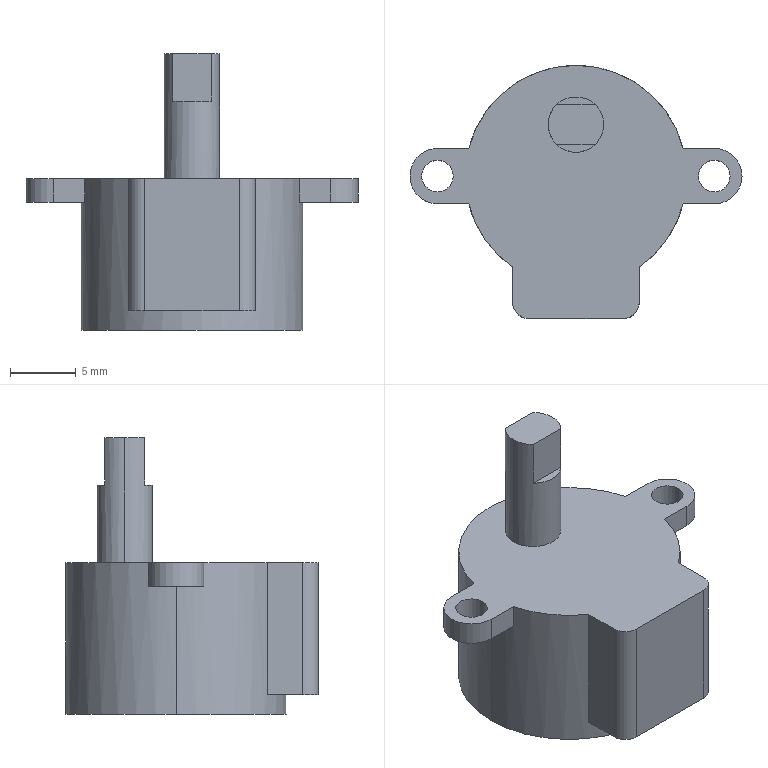Part | SolidWorks | features ICE 4, Extrusion 1, Scale 1 | 1 solid | 30 faces | box 25.2 x 19.2 x 21 mm | volume 2989 mm3 | plane 17 | cylinder 13 | commonest cylinder face diameters 2.4 x6 4.2 x5 16.8 x2
STEP:
#1=CARTESIAN_POINT('',(1.47,5.4,9.48));
#2=VERTEX_POINT('',#1);
#3=CARTESIAN_POINT('',(2.1,3.9,9.48));
#4=VERTEX_POINT('',#3);
#5=CARTESIAN_POINT('',(0.,3.9,9.48));
#6=DIRECTION('',(0.,0.,-1.));
#7=DIRECTION('',(-1.,0.,0.));
#8=AXIS2_PLACEMENT_3D('',#5,#6,#7);
#9=CIRCLE('',#8,2.1);
#10=EDGE_CURVE('',#2,#4,#9,.T.);
#11=ORIENTED_EDGE('',*,*,#10,.T.);
#12=CARTESIAN_POINT('',(2.1,3.9,0.));
#13=VERTEX_POINT('',#12);
#14=CARTESIAN_POINT('',(2.1,3.9,9.48));
#15=DIRECTION('',(0.,0.,-1.));
#16=VECTOR('',#15,1000.);
#17=LINE('',#14,#16);
#18=EDGE_CURVE('',#4,#13,#17,.T.);
#19=ORIENTED_EDGE('',*,*,#18,.T.);
#20=CARTESIAN_POINT('',(-2.1,3.9,0.));
#21=VERTEX_POINT('',#20);
#22=CARTESIAN_POINT('',(0.,3.9,0.));
#23=DIRECTION('',(0.,0.,1.));
#24=DIRECTION('',(1.,0.,0.));
#25=AXIS2_PLACEMENT_3D('',#22,#23,#24);
#26=CIRCLE('',#25,2.1);
#27=EDGE_CURVE('',#13,#21,#26,.T.);
#28=ORIENTED_EDGE('',*,*,#27,.T.);
#29=CARTESIAN_POINT('',(-2.1,3.9,9.48));
#30=VERTEX_POINT('',#29);
#31=CARTESIAN_POINT('',(-2.1,3.9,9.48));
#32=DIRECTION('',(0.,0.,-1.));
#33=VECTOR('',#32,1000.);
#34=LINE('',#31,#33);
#35=EDGE_CURVE('',#30,#21,#34,.T.);
#36=ORIENTED_EDGE('',*,*,#35,.F.);
#37=CARTESIAN_POINT('',(-1.47,5.4,9.48));
#38=VERTEX_POINT('',#37);
#39=CARTESIAN_POINT('',(0.,3.9,9.48));
#40=DIRECTION('',(0.,0.,-1.));
#41=DIRECTION('',(-1.,0.,0.));
#42=AXIS2_PLACEMENT_3D('',#39,#40,#41);
#43=CIRCLE('',#42,2.1);
#44=EDGE_CURVE('',#30,#38,#43,.T.);
#45=ORIENTED_EDGE('',*,*,#44,.T.);
#46=CARTESIAN_POINT('',(-1.47,5.4,5.88));
#47=VERTEX_POINT('',#46);
#48=CARTESIAN_POINT('',(-1.47,5.4,9.48));
#49=DIRECTION('',(0.,0.,1.));
#50=VECTOR('',#49,1000.);
#51=LINE('',#48,#50);
#52=EDGE_CURVE('',#47,#38,#51,.T.);
#53=ORIENTED_EDGE('',*,*,#52,.F.);
#54=CARTESIAN_POINT('',(1.47,5.4,5.88));
#55=VERTEX_POINT('',#54);
#56=CARTESIAN_POINT('',(0.,3.9,5.88));
#57=DIRECTION('',(0.,0.,1.));
#58=DIRECTION('',(-1.,0.,0.));
#59=AXIS2_PLACEMENT_3D('',#56,#57,#58);
#60=CIRCLE('',#59,2.1);
#61=EDGE_CURVE('',#55,#47,#60,.T.);
#62=ORIENTED_EDGE('',*,*,#61,.F.);
#63=CARTESIAN_POINT('',(1.47,5.4,9.48));
#64=DIRECTION('',(0.,0.,-1.));
#65=VECTOR('',#64,1000.);
#66=LINE('',#63,#65);
#67=EDGE_CURVE('',#2,#55,#66,.T.);
#68=ORIENTED_EDGE('',*,*,#67,.F.);
#69=EDGE_LOOP('',(#11,#19,#28,#36,#45,#53,#62,#68));
#70=FACE_OUTER_BOUND('',#69,.T.);
#71=CARTESIAN_POINT('',(0.,3.9,9.48));
#72=DIRECTION('',(0.,0.,-1.));
#73=DIRECTION('',(-1.,0.,0.));
#74=AXIS2_PLACEMENT_3D('',#71,#72,#73);
#75=CYLINDRICAL_SURFACE('',#74,2.1);
#76=ADVANCED_FACE('',(#70),#75,.T.);
#77=CARTESIAN_POINT('',(9.3,0.,-1.8));
#78=VERTEX_POINT('',#77);
#79=CARTESIAN_POINT('',(11.7,0.,-1.8));
#80=VERTEX_POINT('',#79);
#81=CARTESIAN_POINT('',(10.5,0.,-1.8));
#82=DIRECTION('',(0.,0.,1.));
#83=DIRECTION('',(1.,0.,0.));
#84=AXIS2_PLACEMENT_3D('',#81,#82,#83);
#85=CIRCLE('',#84,1.2);
#86=EDGE_CURVE('',#78,#80,#85,.T.);
#87=ORIENTED_EDGE('',*,*,#86,.F.);
#88=CARTESIAN_POINT('',(9.3,0.,0.));
#89=VERTEX_POINT('',#88);
#90=CARTESIAN_POINT('',(9.3,0.,-1.8));
#91=DIRECTION('',(0.,0.,1.));
#92=VECTOR('',#91,1000.);
#93=LINE('',#90,#92);
#94=EDGE_CURVE('',#78,#89,#93,.T.);
#95=ORIENTED_EDGE('',*,*,#94,.T.);
#96=CARTESIAN_POINT('',(11.7,0.,0.));
#97=VERTEX_POINT('',#96);
#98=CARTESIAN_POINT('',(10.5,0.,0.));
#99=DIRECTION('',(0.,0.,1.));
#100=DIRECTION('',(1.,0.,0.));
#101=AXIS2_PLACEMENT_3D('',#98,#99,#100);
#102=CIRCLE('',#101,1.2);
#103=EDGE_CURVE('',#89,#97,#102,.T.);
#104=ORIENTED_EDGE('',*,*,#103,.T.);
#105=CARTESIAN_POINT('',(11.7,0.,-1.8));
#106=DIRECTION('',(0.,0.,1.));
#107=VECTOR('',#106,1000.);
#108=LINE('',#105,#107);
#109=EDGE_CURVE('',#80,#97,#108,.T.);
#110=ORIENTED_EDGE('',*,*,#109,.F.);
#111=EDGE_LOOP('',(#87,#95,#104,#110));
#112=FACE_OUTER_BOUND('',#111,.T.);
#113=CARTESIAN_POINT('',(10.5,0.,-1.8));
#114=DIRECTION('',(0.,0.,1.));
#115=DIRECTION('',(1.,0.,0.));
#116=AXIS2_PLACEMENT_3D('',#113,#114,#115);
#117=CYLINDRICAL_SURFACE('',#116,1.2);
#118=ADVANCED_FACE('',(#112),#117,.F.);
#119=CARTESIAN_POINT('',(10.5,-2.1,-1.8));
#120=VERTEX_POINT('',#119);
#121=CARTESIAN_POINT('',(12.6,0.,-1.8));
#122=VERTEX_POINT('',#121);
#123=CARTESIAN_POINT('',(10.5,0.,-1.8));
#124=DIRECTION('',(0.,0.,1.));
#125=DIRECTION('',(1.,0.,0.));
#126=AXIS2_PLACEMENT_3D('',#123,#124,#125);
#127=CIRCLE('',#126,2.1);
#128=EDGE_CURVE('',#120,#122,#127,.T.);
#129=ORIENTED_EDGE('',*,*,#128,.T.);
#130=CARTESIAN_POINT('',(12.6,0.,0.));
#131=VERTEX_POINT('',#130);
#132=CARTESIAN_POINT('',(12.6,0.,-1.8));
#133=DIRECTION('',(0.,0.,1.));
#134=VECTOR('',#133,1000.);
#135=LINE('',#132,#134);
#136=EDGE_CURVE('',#122,#131,#135,.T.);
#137=ORIENTED_EDGE('',*,*,#136,.T.);
#138=CARTESIAN_POINT('',(10.5,-2.1,0.));
#139=VERTEX_POINT('',#138);
#140=CARTESIAN_POINT('',(10.5,0.,0.));
#141=DIRECTION('',(0.,0.,1.));
#142=DIRECTION('',(1.,0.,0.));
#143=AXIS2_PLACEMENT_3D('',#140,#141,#142);
#144=CIRCLE('',#143,2.1);
#145=EDGE_CURVE('',#139,#131,#144,.T.);
#146=ORIENTED_EDGE('',*,*,#145,.F.);
#147=CARTESIAN_POINT('',(10.5,-2.1,-1.8));
#148=DIRECTION('',(0.,0.,1.));
#149=VECTOR('',#148,1000.);
#150=LINE('',#147,#149);
#151=EDGE_CURVE('',#120,#139,#150,.T.);
#152=ORIENTED_EDGE('',*,*,#151,.F.);
#153=EDGE_LOOP('',(#129,#137,#146,#152));
#154=FACE_OUTER_BOUND('',#153,.T.);
#155=CARTESIAN_POINT('',(10.5,0.,-1.8));
#156=DIRECTION('',(0.,0.,1.));
#157=DIRECTION('',(1.,0.,0.));
#158=AXIS2_PLACEMENT_3D('',#155,#156,#157);
#159=CYLINDRICAL_SURFACE('',#158,2.1);
#160=ADVANCED_FACE('',(#154),#159,.T.);
#161=CARTESIAN_POINT('',(-11.7,0.,-1.8));
#162=VERTEX_POINT('',#161);
#163=CARTESIAN_POINT('',(-9.3,0.,-1.8));
#164=VERTEX_POINT('',#163);
#165=CARTESIAN_POINT('',(-10.5,0.,-1.8));
#166=DIRECTION('',(0.,0.,1.));
#167=DIRECTION('',(1.,0.,0.));
#168=AXIS2_PLACEMENT_3D('',#165,#166,#167);
#169=CIRCLE('',#168,1.2);
#170=EDGE_CURVE('',#162,#164,#169,.T.);
#171=ORIENTED_EDGE('',*,*,#170,.F.);
#172=CARTESIAN_POINT('',(-11.7,0.,0.));
#173=VERTEX_POINT('',#172);
#174=CARTESIAN_POINT('',(-11.7,0.,-1.8));
#175=DIRECTION('',(0.,0.,1.));
#176=VECTOR('',#175,1000.);
#177=LINE('',#174,#176);
#178=EDGE_CURVE('',#162,#173,#177,.T.);
#179=ORIENTED_EDGE('',*,*,#178,.T.);
#180=CARTESIAN_POINT('',(-9.3,0.,0.));
#181=VERTEX_POINT('',#180);
#182=CARTESIAN_POINT('',(-10.5,0.,0.));
#183=DIRECTION('',(0.,0.,1.));
#184=DIRECTION('',(1.,0.,0.));
#185=AXIS2_PLACEMENT_3D('',#182,#183,#184);
#186=CIRCLE('',#185,1.2);
#187=EDGE_CURVE('',#173,#181,#186,.T.);
#188=ORIENTED_EDGE('',*,*,#187,.T.);
#189=CARTESIAN_POINT('',(-9.3,0.,-1.8));
#190=DIRECTION('',(0.,0.,1.));
#191=VECTOR('',#190,1000.);
#192=LINE('',#189,#191);
#193=EDGE_CURVE('',#164,#181,#192,.T.);
#194=ORIENTED_EDGE('',*,*,#193,.F.);
#195=EDGE_LOOP('',(#171,#179,#188,#194));
#196=FACE_OUTER_BOUND('',#195,.T.);
#197=CARTESIAN_POINT('',(-10.5,0.,-1.8));
#198=DIRECTION('',(0.,0.,1.));
#199=DIRECTION('',(1.,0.,0.));
#200=AXIS2_PLACEMENT_3D('',#197,#198,#199);
#201=CYLINDRICAL_SURFACE('',#200,1.2);
#202=ADVANCED_FACE('',(#196),#201,.F.);
#203=CARTESIAN_POINT('',(8.4,0.,-11.52));
#204=VERTEX_POINT('',#203);
#205=CARTESIAN_POINT('',(-8.4,0.,-11.52));
#206=VERTEX_POINT('',#205);
#207=CARTESIAN_POINT('',(0.,0.,-11.52));
#208=DIRECTION('',(0.,0.,1.));
#209=DIRECTION('',(1.,0.,0.));
#210=AXIS2_PLACEMENT_3D('',#207,#208,#209);
#211=CIRCLE('',#210,8.4);
#212=EDGE_CURVE('',#204,#206,#211,.T.);
#213=ORIENTED_EDGE('',*,*,#212,.T.);
#214=CARTESIAN_POINT('',(-8.4,0.,-1.8));
#215=VERTEX_POINT('',#214);
#216=CARTESIAN_POINT('',(-8.4,0.,-11.52));
#217=DIRECTION('',(0.,0.,1.));
#218=VECTOR('',#217,1000.);
#219=LINE('',#216,#218);
#220=EDGE_CURVE('',#206,#215,#219,.T.);
#221=ORIENTED_EDGE('',*,*,#220,.T.);
#222=CARTESIAN_POINT('',(-8.133,2.1,-1.8));
#223=VERTEX_POINT('',#222);
#224=CARTESIAN_POINT('',(0.,0.,-1.8));
#225=DIRECTION('',(0.,0.,1.));
#226=DIRECTION('',(1.,0.,0.));
#227=AXIS2_PLACEMENT_3D('',#224,#225,#226);
#228=CIRCLE('',#227,8.4);
#229=EDGE_CURVE('',#223,#215,#228,.T.);
#230=ORIENTED_EDGE('',*,*,#229,.F.);
#231=CARTESIAN_POINT('',(-8.133,2.1,0.));
#232=VERTEX_POINT('',#231);
#233=CARTESIAN_POINT('',(-8.133,2.1,-1.8));
#234=DIRECTION('',(0.,0.,1.));
#235=VECTOR('',#234,1000.);
#236=LINE('',#233,#235);
#237=EDGE_CURVE('',#223,#232,#236,.T.);
#238=ORIENTED_EDGE('',*,*,#237,.T.);
#239=CARTESIAN_POINT('',(8.133,2.1,0.));
#240=VERTEX_POINT('',#239);
#241=CARTESIAN_POINT('',(0.,0.,0.));
#242=DIRECTION('',(0.,0.,1.));
#243=DIRECTION('',(1.,0.,0.));
#244=AXIS2_PLACEMENT_3D('',#241,#242,#243);
#245=CIRCLE('',#244,8.4);
#246=EDGE_CURVE('',#240,#232,#245,.T.);
#247=ORIENTED_EDGE('',*,*,#246,.F.);
#248=CARTESIAN_POINT('',(8.133,2.1,-1.8));
#249=VERTEX_POINT('',#248);
#250=CARTESIAN_POINT('',(8.133,2.1,-1.8));
#251=DIRECTION('',(0.,0.,1.));
#252=VECTOR('',#251,1000.);
#253=LINE('',#250,#252);
#254=EDGE_CURVE('',#249,#240,#253,.T.);
#255=ORIENTED_EDGE('',*,*,#254,.F.);
#256=CARTESIAN_POINT('',(8.4,0.,-1.8));
#257=VERTEX_POINT('',#256);
#258=CARTESIAN_POINT('',(0.,0.,-1.8));
#259=DIRECTION('',(0.,0.,1.));
#260=DIRECTION('',(1.,0.,0.));
#261=AXIS2_PLACEMENT_3D('',#258,#259,#260);
#262=CIRCLE('',#261,8.4);
#263=EDGE_CURVE('',#257,#249,#262,.T.);
#264=ORIENTED_EDGE('',*,*,#263,.F.);
#265=CARTESIAN_POINT('',(8.4,0.,-11.52));
#266=DIRECTION('',(0.,0.,1.));
#267=VECTOR('',#266,1000.);
#268=LINE('',#265,#267);
#269=EDGE_CURVE('',#204,#257,#268,.T.);
#270=ORIENTED_EDGE('',*,*,#269,.F.);
#271=EDGE_LOOP('',(#213,#221,#230,#238,#247,#255,#264,#270));
#272=FACE_OUTER_BOUND('',#271,.T.);
#273=CARTESIAN_POINT('',(0.,0.,-11.52));
#274=DIRECTION('',(0.,0.,1.));
#275=DIRECTION('',(1.,0.,0.));
#276=AXIS2_PLACEMENT_3D('',#273,#274,#275);
#277=CYLINDRICAL_SURFACE('',#276,8.4);
#278=ADVANCED_FACE('',(#272),#277,.T.);
#279=CARTESIAN_POINT('',(4.8,-6.893,-10.02));
#280=VERTEX_POINT('',#279);
#281=CARTESIAN_POINT('',(4.8,-9.6,-10.02));
#282=VERTEX_POINT('',#281);
#283=CARTESIAN_POINT('',(4.8,-6.893,-10.02));
#284=DIRECTION('',(0.,-1.,0.));
#285=VECTOR('',#284,1000.);
#286=LINE('',#283,#285);
#287=EDGE_CURVE('',#280,#282,#286,.T.);
#288=ORIENTED_EDGE('',*,*,#287,.F.);
#289=CARTESIAN_POINT('',(4.8,-6.893,0.));
#290=VERTEX_POINT('',#289);
#291=CARTESIAN_POINT('',(4.8,-6.893,-11.52));
#292=DIRECTION('',(0.,0.,1.));
#293=VECTOR('',#292,1000.);
#294=LINE('',#291,#293);
#295=EDGE_CURVE('',#280,#290,#294,.T.);
#296=ORIENTED_EDGE('',*,*,#295,.T.);
#297=CARTESIAN_POINT('',(4.8,-9.6,0.));
#298=VERTEX_POINT('',#297);
#299=CARTESIAN_POINT('',(4.8,0.,0.));
#300=DIRECTION('',(0.,-1.,0.));
#301=VECTOR('',#300,1000.);
#302=LINE('',#299,#301);
#303=EDGE_CURVE('',#290,#298,#302,.T.);
#304=ORIENTED_EDGE('',*,*,#303,.T.);
#305=CARTESIAN_POINT('',(4.8,-9.6,-11.52));
#306=DIRECTION('',(0.,0.,1.));
#307=VECTOR('',#306,1000.);
#308=LINE('',#305,#307);
#309=EDGE_CURVE('',#282,#298,#308,.T.);
#310=ORIENTED_EDGE('',*,*,#309,.F.);
#311=EDGE_LOOP('',(#288,#296,#304,#310));
#312=FACE_OUTER_BOUND('',#311,.T.);
#313=CARTESIAN_POINT('',(4.8,0.,-11.52));
#314=DIRECTION('',(-1.,0.,0.));
#315=DIRECTION('',(0.,-1.,0.));
#316=AXIS2_PLACEMENT_3D('',#313,#314,#315);
#317=PLANE('',#316);
#318=ADVANCED_FACE('',(#312),#317,.F.);
#319=CARTESIAN_POINT('',(3.6,-10.8,-10.02));
#320=VERTEX_POINT('',#319);
#321=CARTESIAN_POINT('',(3.6,-9.6,-10.02));
#322=DIRECTION('',(0.,0.,-1.));
#323=DIRECTION('',(-1.,0.,0.));
#324=AXIS2_PLACEMENT_3D('',#321,#322,#323);
#325=CIRCLE('',#324,1.2);
#326=EDGE_CURVE('',#282,#320,#325,.T.);
#327=ORIENTED_EDGE('',*,*,#326,.F.);
#328=ORIENTED_EDGE('',*,*,#309,.T.);
#329=CARTESIAN_POINT('',(3.6,-10.8,0.));
#330=VERTEX_POINT('',#329);
#331=CARTESIAN_POINT('',(3.6,-9.6,0.));
#332=DIRECTION('',(0.,0.,-1.));
#333=DIRECTION('',(1.,0.,0.));
#334=AXIS2_PLACEMENT_3D('',#331,#332,#333);
#335=CIRCLE('',#334,1.2);
#336=EDGE_CURVE('',#298,#330,#335,.T.);
#337=ORIENTED_EDGE('',*,*,#336,.T.);
#338=CARTESIAN_POINT('',(3.6,-10.8,-11.52));
#339=DIRECTION('',(0.,0.,1.));
#340=VECTOR('',#339,1000.);
#341=LINE('',#338,#340);
#342=EDGE_CURVE('',#320,#330,#341,.T.);
#343=ORIENTED_EDGE('',*,*,#342,.F.);
#344=EDGE_LOOP('',(#327,#328,#337,#343));
#345=FACE_OUTER_BOUND('',#344,.T.);
#346=CARTESIAN_POINT('',(3.6,-9.6,-11.52));
#347=DIRECTION('',(0.,0.,1.));
#348=DIRECTION('',(1.,0.,0.));
#349=AXIS2_PLACEMENT_3D('',#346,#347,#348);
#350=CYLINDRICAL_SURFACE('',#349,1.2);
#351=ADVANCED_FACE('',(#345),#350,.T.);
#352=CARTESIAN_POINT('',(-3.6,-10.8,-10.02));
#353=VERTEX_POINT('',#352);
#354=CARTESIAN_POINT('',(-3.6,-10.8,0.));
#355=VERTEX_POINT('',#354);
#356=CARTESIAN_POINT('',(-3.6,-10.8,-11.52));
#357=DIRECTION('',(0.,0.,1.));
#358=VECTOR('',#357,1000.);
#359=LINE('',#356,#358);
#360=EDGE_CURVE('',#353,#355,#359,.T.);
#361=ORIENTED_EDGE('',*,*,#360,.F.);
#362=CARTESIAN_POINT('',(3.6,-10.8,-10.02));
#363=DIRECTION('',(-1.,0.,0.));
#364=VECTOR('',#363,1000.);
#365=LINE('',#362,#364);
#366=EDGE_CURVE('',#320,#353,#365,.T.);
#367=ORIENTED_EDGE('',*,*,#366,.F.);
#368=ORIENTED_EDGE('',*,*,#342,.T.);
#369=CARTESIAN_POINT('',(0.,-10.8,0.));
#370=DIRECTION('',(1.,0.,0.));
#371=VECTOR('',#370,1000.);
#372=LINE('',#369,#371);
#373=EDGE_CURVE('',#355,#330,#372,.T.);
#374=ORIENTED_EDGE('',*,*,#373,.F.);
#375=EDGE_LOOP('',(#361,#367,#368,#374));
#376=FACE_OUTER_BOUND('',#375,.T.);
#377=CARTESIAN_POINT('',(0.,-10.8,-11.52));
#378=DIRECTION('',(0.,-1.,0.));
#379=DIRECTION('',(0.,0.,-1.));
#380=AXIS2_PLACEMENT_3D('',#377,#378,#379);
#381=PLANE('',#380);
#382=ADVANCED_FACE('',(#376),#381,.T.);
#383=CARTESIAN_POINT('',(-4.8,-9.6,-10.02));
#384=VERTEX_POINT('',#383);
#385=CARTESIAN_POINT('',(-4.8,-9.6,0.));
#386=VERTEX_POINT('',#385);
#387=CARTESIAN_POINT('',(-4.8,-9.6,-11.52));
#388=DIRECTION('',(0.,0.,1.));
#389=VECTOR('',#388,1000.);
#390=LINE('',#387,#389);
#391=EDGE_CURVE('',#384,#386,#390,.T.);
#392=ORIENTED_EDGE('',*,*,#391,.F.);
#393=CARTESIAN_POINT('',(-3.6,-9.6,-10.02));
#394=DIRECTION('',(0.,0.,-1.));
#395=DIRECTION('',(-1.,0.,0.));
#396=AXIS2_PLACEMENT_3D('',#393,#394,#395);
#397=CIRCLE('',#396,1.2);
#398=EDGE_CURVE('',#353,#384,#397,.T.);
#399=ORIENTED_EDGE('',*,*,#398,.F.);
#400=ORIENTED_EDGE('',*,*,#360,.T.);
#401=CARTESIAN_POINT('',(-3.6,-9.6,0.));
#402=DIRECTION('',(0.,0.,1.));
#403=DIRECTION('',(1.,0.,0.));
#404=AXIS2_PLACEMENT_3D('',#401,#402,#403);
#405=CIRCLE('',#404,1.2);
#406=EDGE_CURVE('',#386,#355,#405,.T.);
#407=ORIENTED_EDGE('',*,*,#406,.F.);
#408=EDGE_LOOP('',(#392,#399,#400,#407));
#409=FACE_OUTER_BOUND('',#408,.T.);
#410=CARTESIAN_POINT('',(-3.6,-9.6,-11.52));
#411=DIRECTION('',(0.,0.,1.));
#412=DIRECTION('',(1.,0.,0.));
#413=AXIS2_PLACEMENT_3D('',#410,#411,#412);
#414=CYLINDRICAL_SURFACE('',#413,1.2);
#415=ADVANCED_FACE('',(#409),#414,.T.);
#416=CARTESIAN_POINT('',(-4.8,-6.893,-10.02));
#417=VERTEX_POINT('',#416);
#418=CARTESIAN_POINT('',(-4.8,-6.893,0.));
#419=VERTEX_POINT('',#418);
#420=CARTESIAN_POINT('',(-4.8,-6.893,-11.52));
#421=DIRECTION('',(0.,0.,1.));
#422=VECTOR('',#421,1000.);
#423=LINE('',#420,#422);
#424=EDGE_CURVE('',#417,#419,#423,.T.);
#425=ORIENTED_EDGE('',*,*,#424,.F.);
#426=CARTESIAN_POINT('',(-4.8,-9.6,-10.02));
#427=DIRECTION('',(0.,1.,0.));
#428=VECTOR('',#427,1000.);
#429=LINE('',#426,#428);
#430=EDGE_CURVE('',#384,#417,#429,.T.);
#431=ORIENTED_EDGE('',*,*,#430,.F.);
#432=ORIENTED_EDGE('',*,*,#391,.T.);
#433=CARTESIAN_POINT('',(-4.8,0.,0.));
#434=DIRECTION('',(0.,-1.,0.));
#435=VECTOR('',#434,1000.);
#436=LINE('',#433,#435);
#437=EDGE_CURVE('',#419,#386,#436,.T.);
#438=ORIENTED_EDGE('',*,*,#437,.F.);
#439=EDGE_LOOP('',(#425,#431,#432,#438));
#440=FACE_OUTER_BOUND('',#439,.T.);
#441=CARTESIAN_POINT('',(-4.8,0.,-11.52));
#442=DIRECTION('',(-1.,0.,0.));
#443=DIRECTION('',(0.,-1.,0.));
#444=AXIS2_PLACEMENT_3D('',#441,#442,#443);
#445=PLANE('',#444);
#446=ADVANCED_FACE('',(#440),#445,.T.);
#447=ORIENTED_EDGE('',*,*,#220,.F.);
#448=CARTESIAN_POINT('',(0.,0.,-11.52));
#449=DIRECTION('',(0.,0.,1.));
#450=DIRECTION('',(1.,0.,0.));
#451=AXIS2_PLACEMENT_3D('',#448,#449,#450);
#452=CIRCLE('',#451,8.4);
#453=EDGE_CURVE('',#206,#204,#452,.T.);
#454=ORIENTED_EDGE('',*,*,#453,.T.);
#455=ORIENTED_EDGE('',*,*,#269,.T.);
#456=CARTESIAN_POINT('',(8.133,-2.1,-1.8));
#457=VERTEX_POINT('',#456);
#458=CARTESIAN_POINT('',(0.,0.,-1.8));
#459=DIRECTION('',(0.,0.,1.));
#460=DIRECTION('',(1.,0.,0.));
#461=AXIS2_PLACEMENT_3D('',#458,#459,#460);
#462=CIRCLE('',#461,8.4);
#463=EDGE_CURVE('',#457,#257,#462,.T.);
#464=ORIENTED_EDGE('',*,*,#463,.F.);
#465=CARTESIAN_POINT('',(8.133,-2.1,0.));
#466=VERTEX_POINT('',#465);
#467=CARTESIAN_POINT('',(8.133,-2.1,-1.8));
#468=DIRECTION('',(0.,0.,1.));
#469=VECTOR('',#468,1000.);
#470=LINE('',#467,#469);
#471=EDGE_CURVE('',#457,#466,#470,.T.);
#472=ORIENTED_EDGE('',*,*,#471,.T.);
#473=CARTESIAN_POINT('',(0.,0.,0.));
#474=DIRECTION('',(0.,0.,1.));
#475=DIRECTION('',(1.,0.,0.));
#476=AXIS2_PLACEMENT_3D('',#473,#474,#475);
#477=CIRCLE('',#476,8.4);
#478=EDGE_CURVE('',#290,#466,#477,.T.);
#479=ORIENTED_EDGE('',*,*,#478,.F.);
#480=ORIENTED_EDGE('',*,*,#295,.F.);
#481=CARTESIAN_POINT('',(0.,0.,-10.02));
#482=DIRECTION('',(0.,0.,1.));
#483=DIRECTION('',(-1.,0.,0.));
#484=AXIS2_PLACEMENT_3D('',#481,#482,#483);
#485=CIRCLE('',#484,8.4);
#486=EDGE_CURVE('',#417,#280,#485,.T.);
#487=ORIENTED_EDGE('',*,*,#486,.F.);
#488=ORIENTED_EDGE('',*,*,#424,.T.);
#489=CARTESIAN_POINT('',(-8.133,-2.1,0.));
#490=VERTEX_POINT('',#489);
#491=CARTESIAN_POINT('',(0.,0.,0.));
#492=DIRECTION('',(0.,0.,1.));
#493=DIRECTION('',(1.,0.,0.));
#494=AXIS2_PLACEMENT_3D('',#491,#492,#493);
#495=CIRCLE('',#494,8.4);
#496=EDGE_CURVE('',#490,#419,#495,.T.);
#497=ORIENTED_EDGE('',*,*,#496,.F.);
#498=CARTESIAN_POINT('',(-8.133,-2.1,-1.8));
#499=VERTEX_POINT('',#498);
#500=CARTESIAN_POINT('',(-8.133,-2.1,-1.8));
#501=DIRECTION('',(0.,0.,1.));
#502=VECTOR('',#501,1000.);
#503=LINE('',#500,#502);
#504=EDGE_CURVE('',#499,#490,#503,.T.);
#505=ORIENTED_EDGE('',*,*,#504,.F.);
#506=CARTESIAN_POINT('',(0.,0.,-1.8));
#507=DIRECTION('',(0.,0.,1.));
#508=DIRECTION('',(1.,0.,0.));
#509=AXIS2_PLACEMENT_3D('',#506,#507,#508);
#510=CIRCLE('',#509,8.4);
#511=EDGE_CURVE('',#215,#499,#510,.T.);
#512=ORIENTED_EDGE('',*,*,#511,.F.);
#513=EDGE_LOOP('',(#447,#454,#455,#464,#472,#479,#480,#487,#488,#497,#505,#512));
#514=FACE_OUTER_BOUND('',#513,.T.);
#515=CARTESIAN_POINT('',(0.,0.,-11.52));
#516=DIRECTION('',(0.,0.,1.));
#517=DIRECTION('',(1.,0.,0.));
#518=AXIS2_PLACEMENT_3D('',#515,#516,#517);
#519=CYLINDRICAL_SURFACE('',#518,8.4);
#520=ADVANCED_FACE('',(#514),#519,.T.);
#521=ORIENTED_EDGE('',*,*,#212,.F.);
#522=ORIENTED_EDGE('',*,*,#453,.F.);
#523=EDGE_LOOP('',(#521,#522));
#524=FACE_OUTER_BOUND('',#523,.T.);
#525=CARTESIAN_POINT('',(0.,0.,-11.52));
#526=DIRECTION('',(0.,0.,1.));
#527=DIRECTION('',(1.,0.,0.));
#528=AXIS2_PLACEMENT_3D('',#525,#526,#527);
#529=PLANE('',#528);
#530=ADVANCED_FACE('',(#524),#529,.F.);
#531=CARTESIAN_POINT('',(0.,3.9,0.));
#532=DIRECTION('',(0.,0.,1.));
#533=DIRECTION('',(1.,0.,0.));
#534=AXIS2_PLACEMENT_3D('',#531,#532,#533);
#535=CIRCLE('',#534,2.1);
#536=EDGE_CURVE('',#21,#13,#535,.T.);
#537=ORIENTED_EDGE('',*,*,#536,.F.);
#538=ORIENTED_EDGE('',*,*,#27,.F.);
#539=EDGE_LOOP('',(#537,#538));
#540=FACE_BOUND('',#539,.T.);
#541=ORIENTED_EDGE('',*,*,#478,.T.);
#542=CARTESIAN_POINT('',(0.,-2.1,0.));
#543=DIRECTION('',(-1.,0.,0.));
#544=VECTOR('',#543,1000.);
#545=LINE('',#542,#544);
#546=EDGE_CURVE('',#139,#466,#545,.T.);
#547=ORIENTED_EDGE('',*,*,#546,.F.);
#548=ORIENTED_EDGE('',*,*,#145,.T.);
#549=CARTESIAN_POINT('',(10.5,2.1,0.));
#550=VERTEX_POINT('',#549);
#551=CARTESIAN_POINT('',(10.5,0.,0.));
#552=DIRECTION('',(0.,0.,1.));
#553=DIRECTION('',(1.,0.,0.));
#554=AXIS2_PLACEMENT_3D('',#551,#552,#553);
#555=CIRCLE('',#554,2.1);
#556=EDGE_CURVE('',#131,#550,#555,.T.);
#557=ORIENTED_EDGE('',*,*,#556,.T.);
#558=CARTESIAN_POINT('',(0.,2.1,0.));
#559=DIRECTION('',(-1.,0.,0.));
#560=VECTOR('',#559,1000.);
#561=LINE('',#558,#560);
#562=EDGE_CURVE('',#550,#240,#561,.T.);
#563=ORIENTED_EDGE('',*,*,#562,.T.);
#564=ORIENTED_EDGE('',*,*,#246,.T.);
#565=CARTESIAN_POINT('',(-10.5,2.1,0.));
#566=VERTEX_POINT('',#565);
#567=CARTESIAN_POINT('',(0.,2.1,0.));
#568=DIRECTION('',(1.,0.,0.));
#569=VECTOR('',#568,1000.);
#570=LINE('',#567,#569);
#571=EDGE_CURVE('',#566,#232,#570,.T.);
#572=ORIENTED_EDGE('',*,*,#571,.F.);
#573=CARTESIAN_POINT('',(-10.5,-2.1,0.));
#574=VERTEX_POINT('',#573);
#575=CARTESIAN_POINT('',(-10.5,0.,0.));
#576=DIRECTION('',(0.,0.,1.));
#577=DIRECTION('',(1.,0.,0.));
#578=AXIS2_PLACEMENT_3D('',#575,#576,#577);
#579=CIRCLE('',#578,2.1);
#580=EDGE_CURVE('',#566,#574,#579,.T.);
#581=ORIENTED_EDGE('',*,*,#580,.T.);
#582=CARTESIAN_POINT('',(0.,-2.1,0.));
#583=DIRECTION('',(1.,0.,0.));
#584=VECTOR('',#583,1000.);
#585=LINE('',#582,#584);
#586=EDGE_CURVE('',#574,#490,#585,.T.);
#587=ORIENTED_EDGE('',*,*,#586,.T.);
#588=ORIENTED_EDGE('',*,*,#496,.T.);
#589=ORIENTED_EDGE('',*,*,#437,.T.);
#590=ORIENTED_EDGE('',*,*,#406,.T.);
#591=ORIENTED_EDGE('',*,*,#373,.T.);
#592=ORIENTED_EDGE('',*,*,#336,.F.);
#593=ORIENTED_EDGE('',*,*,#303,.F.);
#594=EDGE_LOOP('',(#541,#547,#548,#557,#563,#564,#572,#581,#587,#588,#589,#590,#591,#592,#593));
#595=FACE_OUTER_BOUND('',#594,.T.);
#596=CARTESIAN_POINT('',(-10.5,0.,0.));
#597=DIRECTION('',(0.,0.,1.));
#598=DIRECTION('',(1.,0.,0.));
#599=AXIS2_PLACEMENT_3D('',#596,#597,#598);
#600=CIRCLE('',#599,1.2);
#601=EDGE_CURVE('',#181,#173,#600,.T.);
#602=ORIENTED_EDGE('',*,*,#601,.F.);
#603=ORIENTED_EDGE('',*,*,#187,.F.);
#604=EDGE_LOOP('',(#602,#603));
#605=FACE_BOUND('',#604,.T.);
#606=CARTESIAN_POINT('',(10.5,0.,0.));
#607=DIRECTION('',(0.,0.,1.));
#608=DIRECTION('',(1.,0.,0.));
#609=AXIS2_PLACEMENT_3D('',#606,#607,#608);
#610=CIRCLE('',#609,1.2);
#611=EDGE_CURVE('',#97,#89,#610,.T.);
#612=ORIENTED_EDGE('',*,*,#611,.F.);
#613=ORIENTED_EDGE('',*,*,#103,.F.);
#614=EDGE_LOOP('',(#612,#613));
#615=FACE_BOUND('',#614,.T.);
#616=CARTESIAN_POINT('',(0.,0.,0.));
#617=DIRECTION('',(0.,0.,1.));
#618=DIRECTION('',(1.,0.,0.));
#619=AXIS2_PLACEMENT_3D('',#616,#617,#618);
#620=PLANE('',#619);
#621=ADVANCED_FACE('',(#540,#595,#605,#615),#620,.T.);
#622=ORIENTED_EDGE('',*,*,#586,.F.);
#623=CARTESIAN_POINT('',(-10.5,-2.1,-1.8));
#624=VERTEX_POINT('',#623);
#625=CARTESIAN_POINT('',(-10.5,-2.1,-1.8));
#626=DIRECTION('',(0.,0.,1.));
#627=VECTOR('',#626,1000.);
#628=LINE('',#625,#627);
#629=EDGE_CURVE('',#624,#574,#628,.T.);
#630=ORIENTED_EDGE('',*,*,#629,.F.);
#631=CARTESIAN_POINT('',(0.,-2.1,-1.8));
#632=DIRECTION('',(1.,0.,0.));
#633=VECTOR('',#632,1000.);
#634=LINE('',#631,#633);
#635=EDGE_CURVE('',#624,#499,#634,.T.);
#636=ORIENTED_EDGE('',*,*,#635,.T.);
#637=ORIENTED_EDGE('',*,*,#504,.T.);
#638=EDGE_LOOP('',(#622,#630,#636,#637));
#639=FACE_OUTER_BOUND('',#638,.T.);
#640=CARTESIAN_POINT('',(0.,-2.1,-1.8));
#641=DIRECTION('',(0.,-1.,0.));
#642=DIRECTION('',(1.,0.,0.));
#643=AXIS2_PLACEMENT_3D('',#640,#641,#642);
#644=PLANE('',#643);
#645=ADVANCED_FACE('',(#639),#644,.T.);
#646=ORIENTED_EDGE('',*,*,#580,.F.);
#647=CARTESIAN_POINT('',(-10.5,2.1,-1.8));
#648=VERTEX_POINT('',#647);
#649=CARTESIAN_POINT('',(-10.5,2.1,-1.8));
#650=DIRECTION('',(0.,0.,1.));
#651=VECTOR('',#650,1000.);
#652=LINE('',#649,#651);
#653=EDGE_CURVE('',#648,#566,#652,.T.);
#654=ORIENTED_EDGE('',*,*,#653,.F.);
#655=CARTESIAN_POINT('',(-10.5,0.,-1.8));
#656=DIRECTION('',(0.,0.,1.));
#657=DIRECTION('',(1.,0.,0.));
#658=AXIS2_PLACEMENT_3D('',#655,#656,#657);
#659=CIRCLE('',#658,2.1);
#660=EDGE_CURVE('',#648,#624,#659,.T.);
#661=ORIENTED_EDGE('',*,*,#660,.T.);
#662=ORIENTED_EDGE('',*,*,#629,.T.);
#663=EDGE_LOOP('',(#646,#654,#661,#662));
#664=FACE_OUTER_BOUND('',#663,.T.);
#665=CARTESIAN_POINT('',(-10.5,0.,-1.8));
#666=DIRECTION('',(0.,0.,1.));
#667=DIRECTION('',(1.,0.,0.));
#668=AXIS2_PLACEMENT_3D('',#665,#666,#667);
#669=CYLINDRICAL_SURFACE('',#668,2.1);
#670=ADVANCED_FACE('',(#664),#669,.T.);
#671=ORIENTED_EDGE('',*,*,#571,.T.);
#672=ORIENTED_EDGE('',*,*,#237,.F.);
#673=CARTESIAN_POINT('',(0.,2.1,-1.8));
#674=DIRECTION('',(1.,0.,0.));
#675=VECTOR('',#674,1000.);
#676=LINE('',#673,#675);
#677=EDGE_CURVE('',#648,#223,#676,.T.);
#678=ORIENTED_EDGE('',*,*,#677,.F.);
#679=ORIENTED_EDGE('',*,*,#653,.T.);
#680=EDGE_LOOP('',(#671,#672,#678,#679));
#681=FACE_OUTER_BOUND('',#680,.T.);
#682=CARTESIAN_POINT('',(0.,2.1,-1.8));
#683=DIRECTION('',(0.,-1.,0.));
#684=DIRECTION('',(0.,0.,-1.));
#685=AXIS2_PLACEMENT_3D('',#682,#683,#684);
#686=PLANE('',#685);
#687=ADVANCED_FACE('',(#681),#686,.F.);
#688=ORIENTED_EDGE('',*,*,#178,.F.);
#689=CARTESIAN_POINT('',(-10.5,0.,-1.8));
#690=DIRECTION('',(0.,0.,1.));
#691=DIRECTION('',(1.,0.,0.));
#692=AXIS2_PLACEMENT_3D('',#689,#690,#691);
#693=CIRCLE('',#692,1.2);
#694=EDGE_CURVE('',#164,#162,#693,.T.);
#695=ORIENTED_EDGE('',*,*,#694,.F.);
#696=ORIENTED_EDGE('',*,*,#193,.T.);
#697=ORIENTED_EDGE('',*,*,#601,.T.);
#698=EDGE_LOOP('',(#688,#695,#696,#697));
#699=FACE_OUTER_BOUND('',#698,.T.);
#700=CARTESIAN_POINT('',(-10.5,0.,-1.8));
#701=DIRECTION('',(0.,0.,1.));
#702=DIRECTION('',(1.,0.,0.));
#703=AXIS2_PLACEMENT_3D('',#700,#701,#702);
#704=CYLINDRICAL_SURFACE('',#703,1.2);
#705=ADVANCED_FACE('',(#699),#704,.F.);
#706=ORIENTED_EDGE('',*,*,#229,.T.);
#707=ORIENTED_EDGE('',*,*,#511,.T.);
#708=ORIENTED_EDGE('',*,*,#635,.F.);
#709=ORIENTED_EDGE('',*,*,#660,.F.);
#710=ORIENTED_EDGE('',*,*,#677,.T.);
#711=EDGE_LOOP('',(#706,#707,#708,#709,#710));
#712=FACE_OUTER_BOUND('',#711,.T.);
#713=ORIENTED_EDGE('',*,*,#694,.T.);
#714=ORIENTED_EDGE('',*,*,#170,.T.);
#715=EDGE_LOOP('',(#713,#714));
#716=FACE_BOUND('',#715,.T.);
#717=CARTESIAN_POINT('',(0.,0.,-1.8));
#718=DIRECTION('',(0.,0.,1.));
#719=DIRECTION('',(1.,0.,0.));
#720=AXIS2_PLACEMENT_3D('',#717,#718,#719);
#721=PLANE('',#720);
#722=ADVANCED_FACE('',(#712,#716),#721,.F.);
#723=ORIENTED_EDGE('',*,*,#562,.F.);
#724=CARTESIAN_POINT('',(10.5,2.1,-1.8));
#725=VERTEX_POINT('',#724);
#726=CARTESIAN_POINT('',(10.5,2.1,-1.8));
#727=DIRECTION('',(0.,0.,1.));
#728=VECTOR('',#727,1000.);
#729=LINE('',#726,#728);
#730=EDGE_CURVE('',#725,#550,#729,.T.);
#731=ORIENTED_EDGE('',*,*,#730,.F.);
#732=CARTESIAN_POINT('',(0.,2.1,-1.8));
#733=DIRECTION('',(-1.,0.,0.));
#734=VECTOR('',#733,1000.);
#735=LINE('',#732,#734);
#736=EDGE_CURVE('',#725,#249,#735,.T.);
#737=ORIENTED_EDGE('',*,*,#736,.T.);
#738=ORIENTED_EDGE('',*,*,#254,.T.);
#739=EDGE_LOOP('',(#723,#731,#737,#738));
#740=FACE_OUTER_BOUND('',#739,.T.);
#741=CARTESIAN_POINT('',(0.,2.1,-1.8));
#742=DIRECTION('',(0.,1.,0.));
#743=DIRECTION('',(0.,0.,1.));
#744=AXIS2_PLACEMENT_3D('',#741,#742,#743);
#745=PLANE('',#744);
#746=ADVANCED_FACE('',(#740),#745,.T.);
#747=ORIENTED_EDGE('',*,*,#136,.F.);
#748=CARTESIAN_POINT('',(10.5,0.,-1.8));
#749=DIRECTION('',(0.,0.,1.));
#750=DIRECTION('',(1.,0.,0.));
#751=AXIS2_PLACEMENT_3D('',#748,#749,#750);
#752=CIRCLE('',#751,2.1);
#753=EDGE_CURVE('',#122,#725,#752,.T.);
#754=ORIENTED_EDGE('',*,*,#753,.T.);
#755=ORIENTED_EDGE('',*,*,#730,.T.);
#756=ORIENTED_EDGE('',*,*,#556,.F.);
#757=EDGE_LOOP('',(#747,#754,#755,#756));
#758=FACE_OUTER_BOUND('',#757,.T.);
#759=CARTESIAN_POINT('',(10.5,0.,-1.8));
#760=DIRECTION('',(0.,0.,1.));
#761=DIRECTION('',(1.,0.,0.));
#762=AXIS2_PLACEMENT_3D('',#759,#760,#761);
#763=CYLINDRICAL_SURFACE('',#762,2.1);
#764=ADVANCED_FACE('',(#758),#763,.T.);
#765=ORIENTED_EDGE('',*,*,#546,.T.);
#766=ORIENTED_EDGE('',*,*,#471,.F.);
#767=CARTESIAN_POINT('',(0.,-2.1,-1.8));
#768=DIRECTION('',(-1.,0.,0.));
#769=VECTOR('',#768,1000.);
#770=LINE('',#767,#769);
#771=EDGE_CURVE('',#120,#457,#770,.T.);
#772=ORIENTED_EDGE('',*,*,#771,.F.);
#773=ORIENTED_EDGE('',*,*,#151,.T.);
#774=EDGE_LOOP('',(#765,#766,#772,#773));
#775=FACE_OUTER_BOUND('',#774,.T.);
#776=CARTESIAN_POINT('',(0.,-2.1,-1.8));
#777=DIRECTION('',(0.,1.,0.));
#778=DIRECTION('',(0.,0.,1.));
#779=AXIS2_PLACEMENT_3D('',#776,#777,#778);
#780=PLANE('',#779);
#781=ADVANCED_FACE('',(#775),#780,.F.);
#782=ORIENTED_EDGE('',*,*,#94,.F.);
#783=CARTESIAN_POINT('',(10.5,0.,-1.8));
#784=DIRECTION('',(0.,0.,1.));
#785=DIRECTION('',(1.,0.,0.));
#786=AXIS2_PLACEMENT_3D('',#783,#784,#785);
#787=CIRCLE('',#786,1.2);
#788=EDGE_CURVE('',#80,#78,#787,.T.);
#789=ORIENTED_EDGE('',*,*,#788,.F.);
#790=ORIENTED_EDGE('',*,*,#109,.T.);
#791=ORIENTED_EDGE('',*,*,#611,.T.);
#792=EDGE_LOOP('',(#782,#789,#790,#791));
#793=FACE_OUTER_BOUND('',#792,.T.);
#794=CARTESIAN_POINT('',(10.5,0.,-1.8));
#795=DIRECTION('',(0.,0.,1.));
#796=DIRECTION('',(1.,0.,0.));
#797=AXIS2_PLACEMENT_3D('',#794,#795,#796);
#798=CYLINDRICAL_SURFACE('',#797,1.2);
#799=ADVANCED_FACE('',(#793),#798,.F.);
#800=ORIENTED_EDGE('',*,*,#463,.T.);
#801=ORIENTED_EDGE('',*,*,#263,.T.);
#802=ORIENTED_EDGE('',*,*,#736,.F.);
#803=ORIENTED_EDGE('',*,*,#753,.F.);
#804=ORIENTED_EDGE('',*,*,#128,.F.);
#805=ORIENTED_EDGE('',*,*,#771,.T.);
#806=EDGE_LOOP('',(#800,#801,#802,#803,#804,#805));
#807=FACE_OUTER_BOUND('',#806,.T.);
#808=ORIENTED_EDGE('',*,*,#788,.T.);
#809=ORIENTED_EDGE('',*,*,#86,.T.);
#810=EDGE_LOOP('',(#808,#809));
#811=FACE_BOUND('',#810,.T.);
#812=CARTESIAN_POINT('',(0.,0.,-1.8));
#813=DIRECTION('',(0.,0.,1.));
#814=DIRECTION('',(1.,0.,0.));
#815=AXIS2_PLACEMENT_3D('',#812,#813,#814);
#816=PLANE('',#815);
#817=ADVANCED_FACE('',(#807,#811),#816,.F.);
#818=ORIENTED_EDGE('',*,*,#10,.F.);
#819=CARTESIAN_POINT('',(-3.,5.4,9.48));
#820=DIRECTION('',(1.,0.,0.));
#821=VECTOR('',#820,1000.);
#822=LINE('',#819,#821);
#823=EDGE_CURVE('',#38,#2,#822,.T.);
#824=ORIENTED_EDGE('',*,*,#823,.F.);
#825=ORIENTED_EDGE('',*,*,#44,.F.);
#826=CARTESIAN_POINT('',(-1.47,2.4,9.48));
#827=VERTEX_POINT('',#826);
#828=CARTESIAN_POINT('',(0.,3.9,9.48));
#829=DIRECTION('',(0.,0.,-1.));
#830=DIRECTION('',(-1.,0.,0.));
#831=AXIS2_PLACEMENT_3D('',#828,#829,#830);
#832=CIRCLE('',#831,2.1);
#833=EDGE_CURVE('',#827,#30,#832,.T.);
#834=ORIENTED_EDGE('',*,*,#833,.F.);
#835=CARTESIAN_POINT('',(1.47,2.4,9.48));
#836=VERTEX_POINT('',#835);
#837=CARTESIAN_POINT('',(-3.,2.4,9.48));
#838=DIRECTION('',(1.,0.,0.));
#839=VECTOR('',#838,1000.);
#840=LINE('',#837,#839);
#841=EDGE_CURVE('',#827,#836,#840,.T.);
#842=ORIENTED_EDGE('',*,*,#841,.T.);
#843=CARTESIAN_POINT('',(0.,3.9,9.48));
#844=DIRECTION('',(0.,0.,-1.));
#845=DIRECTION('',(-1.,0.,0.));
#846=AXIS2_PLACEMENT_3D('',#843,#844,#845);
#847=CIRCLE('',#846,2.1);
#848=EDGE_CURVE('',#4,#836,#847,.T.);
#849=ORIENTED_EDGE('',*,*,#848,.F.);
#850=EDGE_LOOP('',(#818,#824,#825,#834,#842,#849));
#851=FACE_OUTER_BOUND('',#850,.T.);
#852=CARTESIAN_POINT('',(0.,3.9,9.48));
#853=DIRECTION('',(0.,0.,-1.));
#854=DIRECTION('',(-1.,0.,0.));
#855=AXIS2_PLACEMENT_3D('',#852,#853,#854);
#856=PLANE('',#855);
#857=ADVANCED_FACE('',(#851),#856,.F.);
#858=ORIENTED_EDGE('',*,*,#18,.F.);
#859=ORIENTED_EDGE('',*,*,#848,.T.);
#860=CARTESIAN_POINT('',(1.47,2.4,5.88));
#861=VERTEX_POINT('',#860);
#862=CARTESIAN_POINT('',(1.47,2.4,9.48));
#863=DIRECTION('',(0.,0.,1.));
#864=VECTOR('',#863,1000.);
#865=LINE('',#862,#864);
#866=EDGE_CURVE('',#861,#836,#865,.T.);
#867=ORIENTED_EDGE('',*,*,#866,.F.);
#868=CARTESIAN_POINT('',(-1.47,2.4,5.88));
#869=VERTEX_POINT('',#868);
#870=CARTESIAN_POINT('',(0.,3.9,5.88));
#871=DIRECTION('',(0.,0.,1.));
#872=DIRECTION('',(-1.,0.,0.));
#873=AXIS2_PLACEMENT_3D('',#870,#871,#872);
#874=CIRCLE('',#873,2.1);
#875=EDGE_CURVE('',#869,#861,#874,.T.);
#876=ORIENTED_EDGE('',*,*,#875,.F.);
#877=CARTESIAN_POINT('',(-1.47,2.4,9.48));
#878=DIRECTION('',(0.,0.,-1.));
#879=VECTOR('',#878,1000.);
#880=LINE('',#877,#879);
#881=EDGE_CURVE('',#827,#869,#880,.T.);
#882=ORIENTED_EDGE('',*,*,#881,.F.);
#883=ORIENTED_EDGE('',*,*,#833,.T.);
#884=ORIENTED_EDGE('',*,*,#35,.T.);
#885=ORIENTED_EDGE('',*,*,#536,.T.);
#886=EDGE_LOOP('',(#858,#859,#867,#876,#882,#883,#884,#885));
#887=FACE_OUTER_BOUND('',#886,.T.);
#888=CARTESIAN_POINT('',(0.,3.9,9.48));
#889=DIRECTION('',(0.,0.,-1.));
#890=DIRECTION('',(-1.,0.,0.));
#891=AXIS2_PLACEMENT_3D('',#888,#889,#890);
#892=CYLINDRICAL_SURFACE('',#891,2.1);
#893=ADVANCED_FACE('',(#887),#892,.T.);
#894=ORIENTED_EDGE('',*,*,#486,.T.);
#895=ORIENTED_EDGE('',*,*,#287,.T.);
#896=ORIENTED_EDGE('',*,*,#326,.T.);
#897=ORIENTED_EDGE('',*,*,#366,.T.);
#898=ORIENTED_EDGE('',*,*,#398,.T.);
#899=ORIENTED_EDGE('',*,*,#430,.T.);
#900=EDGE_LOOP('',(#894,#895,#896,#897,#898,#899));
#901=FACE_OUTER_BOUND('',#900,.T.);
#902=CARTESIAN_POINT('',(0.,0.,-10.02));
#903=DIRECTION('',(0.,0.,-1.));
#904=DIRECTION('',(-1.,0.,0.));
#905=AXIS2_PLACEMENT_3D('',#902,#903,#904);
#906=PLANE('',#905);
#907=ADVANCED_FACE('',(#901),#906,.T.);
#908=ORIENTED_EDGE('',*,*,#866,.T.);
#909=ORIENTED_EDGE('',*,*,#841,.F.);
#910=ORIENTED_EDGE('',*,*,#881,.T.);
#911=CARTESIAN_POINT('',(-3.,2.4,5.88));
#912=DIRECTION('',(1.,0.,0.));
#913=VECTOR('',#912,1000.);
#914=LINE('',#911,#913);
#915=EDGE_CURVE('',#869,#861,#914,.T.);
#916=ORIENTED_EDGE('',*,*,#915,.T.);
#917=EDGE_LOOP('',(#908,#909,#910,#916));
#918=FACE_OUTER_BOUND('',#917,.T.);
#919=CARTESIAN_POINT('',(-3.,2.4,9.48));
#920=DIRECTION('',(0.,1.,0.));
#921=DIRECTION('',(0.,0.,1.));
#922=AXIS2_PLACEMENT_3D('',#919,#920,#921);
#923=PLANE('',#922);
#924=ADVANCED_FACE('',(#918),#923,.F.);
#925=ORIENTED_EDGE('',*,*,#915,.F.);
#926=ORIENTED_EDGE('',*,*,#875,.T.);
#927=EDGE_LOOP('',(#925,#926));
#928=FACE_OUTER_BOUND('',#927,.T.);
#929=CARTESIAN_POINT('',(-3.,1.8,5.88));
#930=DIRECTION('',(0.,0.,-1.));
#931=DIRECTION('',(-1.,0.,0.));
#932=AXIS2_PLACEMENT_3D('',#929,#930,#931);
#933=PLANE('',#932);
#934=ADVANCED_FACE('',(#928),#933,.F.);
#935=ORIENTED_EDGE('',*,*,#61,.T.);
#936=CARTESIAN_POINT('',(-3.,5.4,5.88));
#937=DIRECTION('',(1.,0.,0.));
#938=VECTOR('',#937,1000.);
#939=LINE('',#936,#938);
#940=EDGE_CURVE('',#47,#55,#939,.T.);
#941=ORIENTED_EDGE('',*,*,#940,.T.);
#942=EDGE_LOOP('',(#935,#941));
#943=FACE_OUTER_BOUND('',#942,.T.);
#944=CARTESIAN_POINT('',(-3.,6.,5.88));
#945=DIRECTION('',(0.,0.,-1.));
#946=DIRECTION('',(-1.,0.,0.));
#947=AXIS2_PLACEMENT_3D('',#944,#945,#946);
#948=PLANE('',#947);
#949=ADVANCED_FACE('',(#943),#948,.F.);
#950=ORIENTED_EDGE('',*,*,#52,.T.);
#951=ORIENTED_EDGE('',*,*,#823,.T.);
#952=ORIENTED_EDGE('',*,*,#67,.T.);
#953=ORIENTED_EDGE('',*,*,#940,.F.);
#954=EDGE_LOOP('',(#950,#951,#952,#953));
#955=FACE_OUTER_BOUND('',#954,.T.);
#956=CARTESIAN_POINT('',(-3.,5.4,9.48));
#957=DIRECTION('',(0.,-1.,0.));
#958=DIRECTION('',(0.,0.,-1.));
#959=AXIS2_PLACEMENT_3D('',#956,#957,#958);
#960=PLANE('',#959);
#961=ADVANCED_FACE('',(#955),#960,.F.);
#962=CLOSED_SHELL('',(#76,#118,#160,#202,#278,#318,#351,#382,#415,#446,#520,#530,#621,#645,#670,#687,#705,#722,#746,#764,#781,#799,#817,#857,#893,#907,#924,#934,#949,#961));
#963=MANIFOLD_SOLID_BREP('',#962);
#964=CARTESIAN_POINT('',(0.,0.,0.));
#965=DIRECTION('',(0.,0.,1.));
#966=DIRECTION('',(1.,0.,0.));
#967=AXIS2_PLACEMENT_3D('',#964,#965,#966);
#968=(LENGTH_UNIT()NAMED_UNIT(*)SI_UNIT(.MILLI.,.METRE.));
#969=UNCERTAINTY_MEASURE_WITH_UNIT(LENGTH_MEASURE(0.00001),#968,'','');
#970=(NAMED_UNIT(*)PLANE_ANGLE_UNIT()SI_UNIT($,.RADIAN.));
#971=(NAMED_UNIT(*)SI_UNIT($,.STERADIAN.)SOLID_ANGLE_UNIT());
#972=(GEOMETRIC_REPRESENTATION_CONTEXT(3)GLOBAL_UNCERTAINTY_ASSIGNED_CONTEXT((#969))GLOBAL_UNIT_ASSIGNED_CONTEXT((#968,#970,#971))REPRESENTATION_CONTEXT('',''));
#973=ADVANCED_BREP_SHAPE_REPRESENTATION('',(#963,#967),#972);